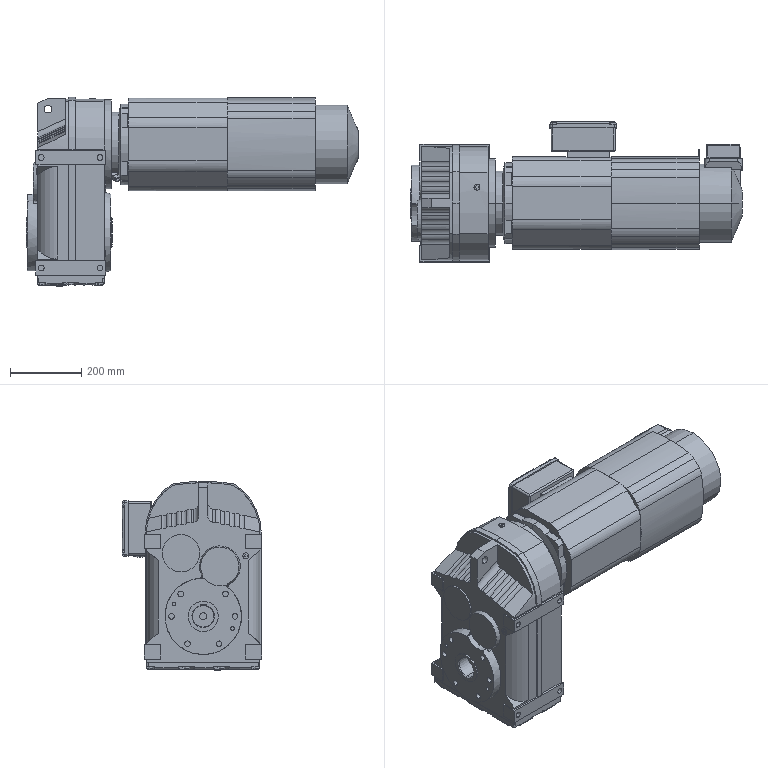Part | SolidWorks | features BaseBody 1 | 1 solid | 822 faces | box 932 x 393 x 531.376 mm | volume 69762381 mm3 | plane 476 | cylinder 294 | spline 38 | cone 14 | commonest cylinder face diameters 0.2 x31 16 x28 34 x22 8 x18 4 x13 5 x12